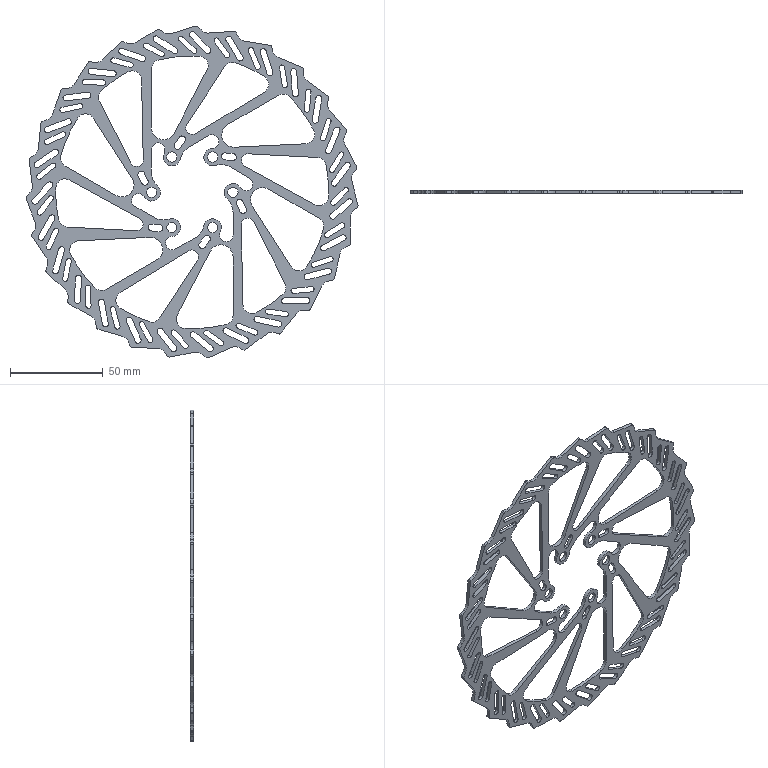Part | SolidWorks | features BaseBody 1 | 1 solid | 545 faces | box 179.47 x 1.84 x 179.441 mm | volume 17424 mm3 | cylinder 333 | plane 212 | commonest cylinder face diameters 2.783 x81 3.243 x81 10 x60 179.78 x27 3.718 x18 147.478 x13